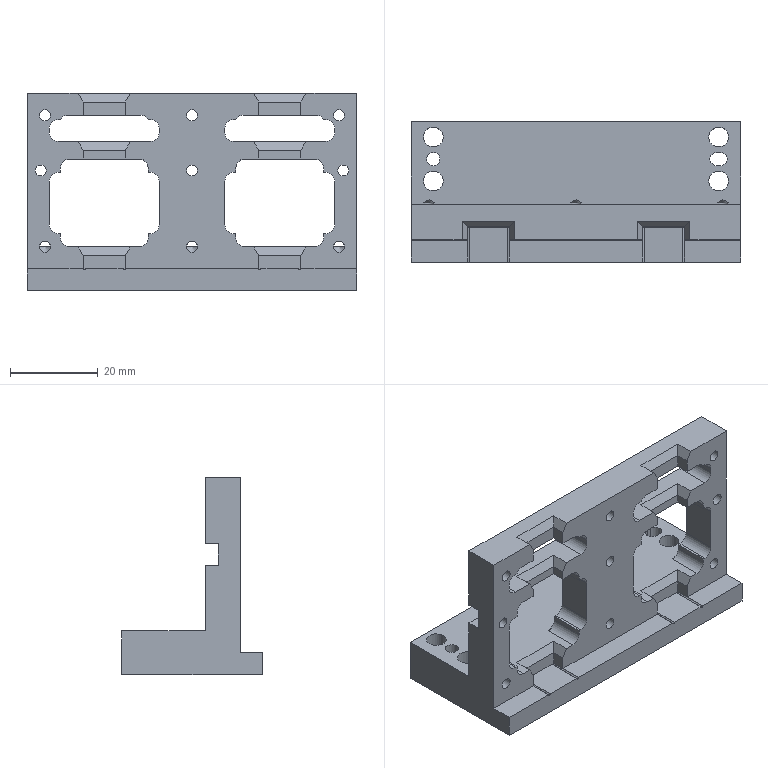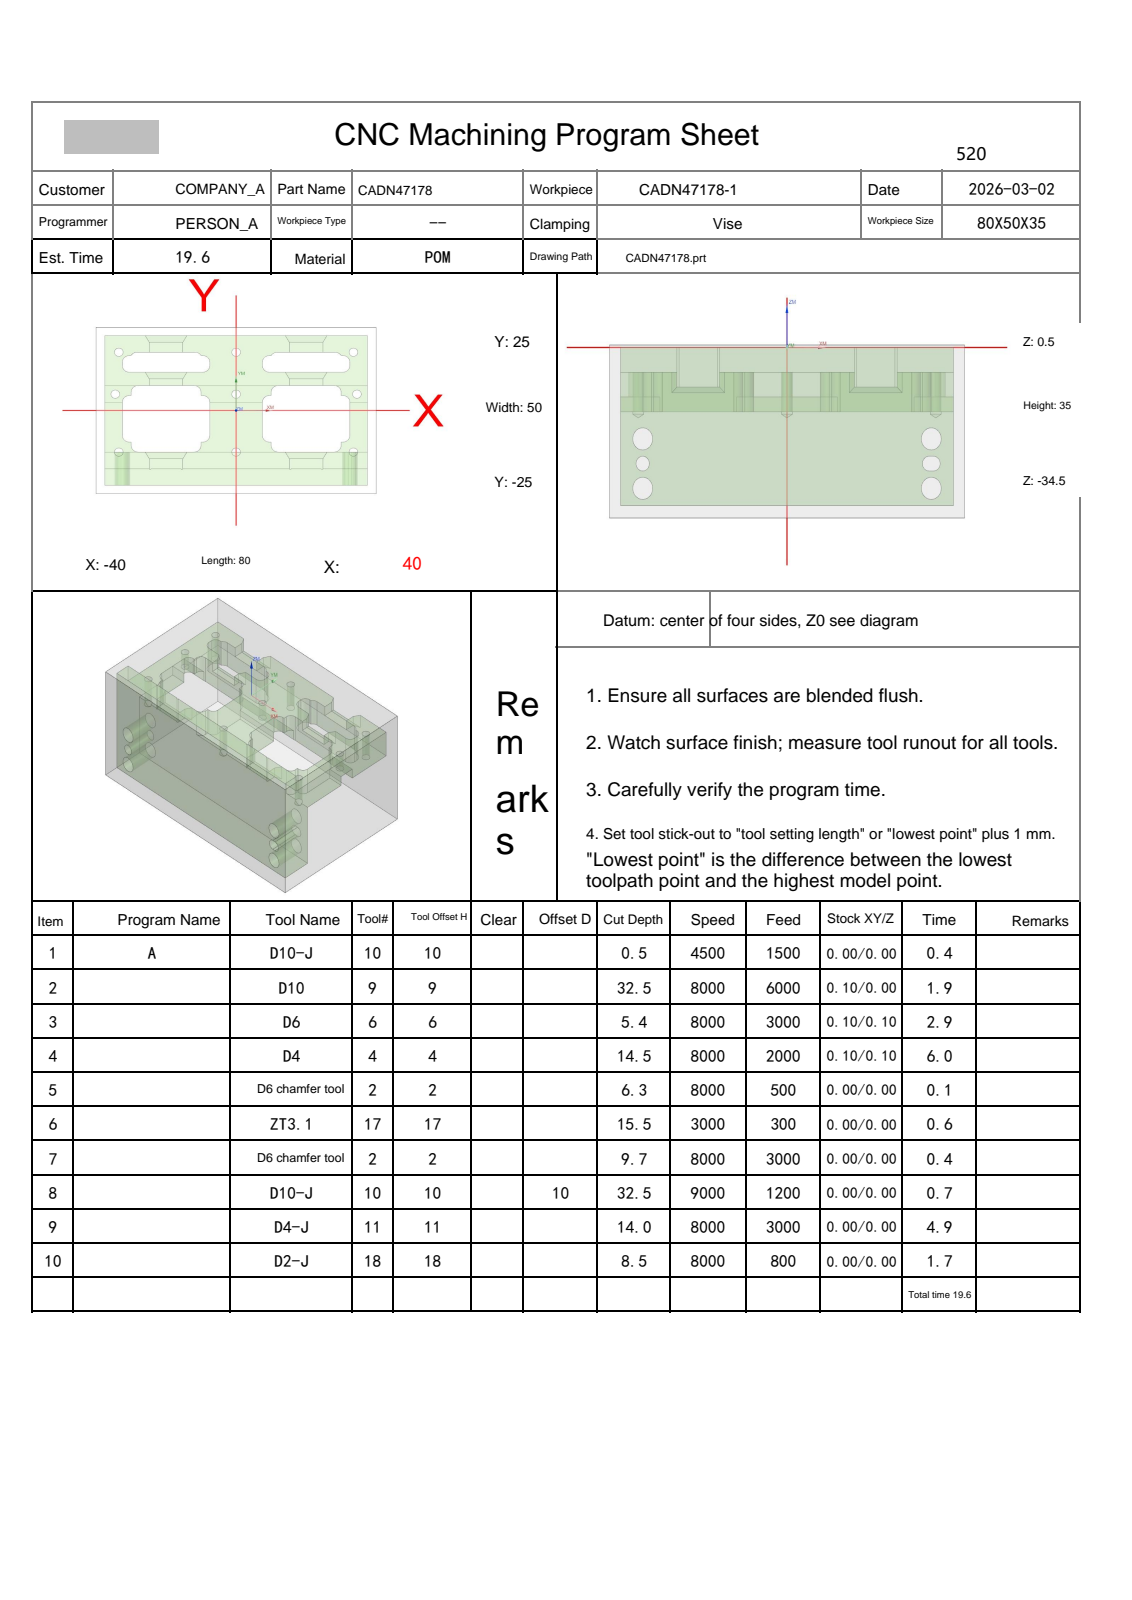NC program | NX | posted by the shop | part box 75 x 32 x 45 mm
Lines 8500 to 9882 of 18359:
N9 T11 M06
(D4-J  D=4. R=0. H=11 ce=0.40 di=0.00)
G00 G90 G54 X-40.3 Y7.17 M03 S7000
G43 H11 Z10.5
M08
Z-3.5
G01 Z-5. F1500.
X-38.7
G03 X-37.9 Y7.97 I0.0 J.8
G01 Y22.501
G02 X-37.501 Y22.9 I.4 J-.001
G01 X-25.954
G02 X-25.609 Y22.701 I-.001 J-.4
G01 X-24.453 Y20.699
G02 X-24.4 Y20.501 I-.347 J-.199
G01 Y17.499
G02 X-24.799 Y17.1 I-.4 J.001
G01 X-29.192
X-29.654 Y16.299
G02 X-29.999 Y16.1 I-.346 J.201
G01 X-32.1
Y11.9
X-25.954
G02 X-25.609 Y11.701 I-.001 J-.4
G01 X-24.453 Y9.699
G02 X-24.4 Y9.501 I-.347 J-.199
G01 Y7.499
G02 X-24.799 Y7.1 I-.4 J.001
G01 X-29.6
Y4.499
G02 X-29.999 Y4.1 I-.4 J.001
G01 X-32.1
Y-9.1
X-29.999
G02 X-29.6 Y-9.499 I-.001 J-.4
G01 Y-12.1
X-25.954
G02 X-25.609 Y-12.299 I-.001 J-.4
G01 X-24.453 Y-14.301
G02 X-24.4 Y-14.499 I-.347 J-.199
G01 Y-14.701
G02 X-24.799 Y-15.1 I-.4 J.001
G01 X-37.501
G02 X-37.9 Y-14.701 I.001 J.4
G01 Y8.805
G02 X-37.783 Y9.087 I.4 J0.0
G01 X-36.017 Y10.853
G03 X-35.9 Y11.135 I-.283 J.283
G01 Y20.501
G02 X-35.501 Y20.9 I.4 J-.001
G01 X-27.108
G02 X-26.764 Y20.701 I-.001 J-.4
G01 X-26.453 Y20.163
G02 X-26.4 Y19.965 I-.347 J-.199
G01 Y19.499
G02 X-26.799 Y19.1 I-.4 J.001
G01 X-29.192
G03 X-30.817 Y18.266 I0.0 J-2.
G02 X-31.14 Y18.1 I-.324 J.234
G01 X-32.1
G03 X-34.1 Y16.1 I0.0 J-2.
G01 Y11.9
G03 X-32.1 Y9.9 I2. J0.0
G01 X-27.108
G02 X-26.709 Y9.5 I-.001 J-.4
X-27.108 Y9.1 I-.4 J0.0
G01 X-29.6
G03 X-31.6 Y7.1 I0.0 J-2.
G01 Y6.499
G02 X-31.999 Y6.1 I-.4 J.001
G01 X-32.1
G03 X-34.1 Y4.1 I0.0 J-2.
G01 Y-9.1
G03 X-32.1 Y-11.1 I2. J0.0
G01 X-31.999
G02 X-31.6 Y-11.499 I-.001 J-.4
G01 Y-12.1
G03 X-31.536 Y-12.601 I2. J0.0
G01 X-31.524 Y-12.7
G02 X-31.923 Y-13.1 I-.4 J0.0
G01 X-35.501
G02 X-35.9 Y-12.701 I.001 J.4
G01 Y8.615
G02 X-35.66 Y8.855 I.24 J0.0
G01 X-35.571 Y8.838
X-34.132 Y8.263
G03 X-33.841 Y8.207 I.291 J.729
G01 X-33.729 Y8.215
X-33.673 Y8.225
X-33.622 Y8.201
G02 X-33.499 Y8.016 I-.077 J-.185
G01 X-33.503 Y7.973
X-33.515 Y7.918
X-33.526 Y7.865
X-33.56 Y7.823
X-33.611 Y7.804
X-33.678 Y7.776
X-33.74 Y7.763
G02 X-33.9 Y7.922 I0.0 J.16
G01 Y8.018
X-33.904 Y8.068
X-33.886 Y8.115
X-33.85 Y8.149
X-33.7 Y8.217
X-33.622 Y8.201
G02 X-33.499 Y8.016 I-.077 J-.185
G01 X-33.503 Y7.973
X-33.515 Y7.918
X-33.526 Y7.865
X-33.56 Y7.823
X-33.611 Y7.804
X-33.678 Y7.776
X-33.739 Y7.753
X-33.804 Y7.766
X-33.852 Y7.809
G03 X-34.414 Y8.039 I-.561 J-.57
X-34.984 Y7.801 I0.0 J-.8
G01 Z-3.5
G00 Z-1.
X11.818 Y14.3
Z-3.5
G01 Z-5.
X8.7 Y12.7
G03 X7.9 Y11.9 I0.0 J-.8
G01 X14.047
G02 X14.392 Y11.7 I-.001 J-.4
G01 X15.547 Y9.699
G02 X15.6 Y9.501 I-.347 J-.199
G01 Y7.499
G02 X15.201 Y7.1 I-.4 J.001
G01 X10.4
Y4.345
G02 X10.2 Y4.146 I-.2 J.001
G01 X10.059 Y4.204
X9.875 Y4.387
X7.9 Y3.569
Y-9.1
X10.001
G02 X10.4 Y-9.499 I-.001 J-.4
G01 Y-12.1
X14.047
G02 X14.391 Y-12.299 I-.001 J-.4
G01 X15.547 Y-14.301
G02 X15.6 Y-14.499 I-.347 J-.199
G01 Y-14.701
G02 X15.201 Y-15.1 I-.4 J.001
G01 X-15.201
G02 X-15.6 Y-14.701 I.001 J.4
G01 Y-14.499
G02 X-15.547 Y-14.301 I.4 J-.001
G01 X-14.391 Y-12.299
G02 X-14.047 Y-12.1 I.346 J-.201
G01 X-10.4
Y-9.499
G02 X-10.001 Y-9.1 I.4 J-.001
G01 X-7.9
Y3.489
X-9.122 Y4.1
X-10.001
G02 X-10.4 Y4.499 I.001 J.4
G01 Y7.1
X-15.201
G02 X-15.6 Y7.499 I.001 J.4
G01 Y9.501
G02 X-15.547 Y9.699 I.4 J-.001
G01 X-14.391 Y11.701
G02 X-14.047 Y11.9 I.346 J-.201
G01 X-7.9
Y16.1
X-10.001
G02 X-10.346 Y16.299 I.001 J.4
G01 X-10.808 Y17.1
X-15.201
G02 X-15.6 Y17.499 I.001 J.4
G01 Y20.501
G02 X-15.547 Y20.699 I.4 J-.001
G01 X-14.391 Y22.701
G02 X-14.047 Y22.9 I.346 J-.201
G01 X14.047
G02 X14.391 Y22.701 I-.001 J-.4
G01 X15.547 Y20.699
G02 X15.6 Y20.501 I-.347 J-.199
G01 Y17.499
G02 X15.201 Y17.1 I-.4 J.001
G01 X10.808
X10.346 Y16.299
G02 X10.001 Y16.1 I-.346 J.201
G01 X7.9
Y11.9
X9.9
G02 X10.276 Y11.635 I0.0 J-.4
G01 X10.805 Y10.165
G03 X11.181 Y9.9 I.376 J.135
G01 X12.892
G02 X13.291 Y9.5 I-.001 J-.4
X12.892 Y9.1 I-.4 J0.0
G01 X10.4
G03 X8.4 Y7.1 I0.0 J-2.
G01 Y6.207
G02 X8.154 Y5.839 I-.4 J.001
G01 X7.135 Y5.417
G03 X5.9 Y3.569 I.765 J-1.848
G01 Y-9.1
G03 X7.9 Y-11.1 I2. J0.0
G01 X8.001
G02 X8.4 Y-11.499 I-.001 J-.4
G01 Y-12.1
G03 X8.464 Y-12.601 I2. J0.0
G01 X8.476 Y-12.7
G02 X8.078 Y-13.1 I-.4 J0.0
G01 X-8.078
G02 X-8.476 Y-12.7 I.001 J.4
G01 X-8.464 Y-12.601
G03 X-8.4 Y-12.1 I-1.936 J.501
G01 Y-11.499
G02 X-8.001 Y-11.1 I.4 J-.001
G01 X-7.9
G03 X-5.9 Y-9.1 I0.0 J2.
G01 Y3.489
G03 X-7.006 Y5.278 I-2. J0.0
G01 X-8.18 Y5.865
G02 X-8.4 Y6.221 I.18 J.357
G01 Y7.1
G03 X-10.4 Y9.1 I-2. J0.0
G01 X-12.892
G02 X-13.291 Y9.5 I.001 J.4
X-12.892 Y9.9 I.4 J0.0
G01 X-7.9
G03 X-5.9 Y11.9 I0.0 J2.
G01 Y16.1
G03 X-7.9 Y18.1 I-2. J0.0
G01 X-8.86
G02 X-9.183 Y18.266 I.001 J.4
G03 X-10.808 Y19.1 I-1.625 J-1.166
G01 X-13.201
G02 X-13.6 Y19.499 I.001 J.4
G01 Y19.965
G02 X-13.547 Y20.163 I.4 J-.001
G01 X-13.236 Y20.701
G02 X-12.892 Y20.9 I.346 J-.201
G01 X12.892
G02 X13.236 Y20.701 I-.001 J-.4
G01 X13.547 Y20.163
G02 X13.6 Y19.965 I-.347 J-.199
G01 Y19.499
G02 X13.201 Y19.1 I-.4 J.001
G01 X10.808
G03 X9.183 Y18.266 I0.0 J-2.
G02 X8.86 Y18.1 I-.324 J.234
G01 X7.9
G03 X5.9 Y16.1 I0.0 J-2.
G01 Y11.9
G03 X7.9 Y9.9 I2. J0.0
G01 X8.504
G02 X8.664 Y9.74 I0.0 J-.16
G01 X8.615 Y9.625
X6.506 Y7.588
X6.455 Y7.546
X6.419 Y7.489
X6.403 Y7.425
G02 X6.195 Y7.187 I-.38 J.124
G03 X3.9 Y3.569 I1.705 J-3.618
G01 Y-9.1
G03 X4.174 Y-10.556 I4. J0.0
G01 X4.201 Y-10.7
G02 X3.803 Y-11.1 I-.4 J0.0
G01 X-3.803
G02 X-4.201 Y-10.7 I.001 J.4
G01 X-4.174 Y-10.556
G03 X-3.9 Y-9.1 I-3.726 J1.456
G01 Y3.489
G03 X-6.111 Y7.067 I-4. J0.0
G01 X-6.195 Y7.109
G02 X-6.414 Y7.431 I.18 J.357
G03 X-6.466 Y7.826 I-3.986 J-.331
G01 X-6.473 Y7.897
G02 X-6.24 Y8.261 I.4 J0.0
G03 X-3.9 Y11.9 I-1.66 J3.639
G01 Y16.1
G03 X-4.548 Y18.283 I-4. J0.0
G02 X-4.612 Y18.5 I.336 J.217
X-4.214 Y18.9 I.4 J0.0
G01 X4.214
G02 X4.612 Y18.5 I-.001 J-.4
X4.548 Y18.283 I-.4 J0.0
G03 X3.9 Y16.1 I3.352 J-2.183
G01 Y11.9
G03 X5.297 Y8.862 I4. J0.0
G02 X5.395 Y8.65 I-.182 J-.213
X5.265 Y8.413 I-.28 J0.0
G01 X3.006 Y6.983
X2.933 Y6.937
X2.886 Y6.865
G03 X1.9 Y3.569 I5.014 J-3.296
G01 Y-8.702
G02 X1.502 Y-9.1 I-.4 J.002
G01 X-1.502
G02 X-1.9 Y-8.702 I.002 J.4
G01 Y3.489
G03 X-3.378 Y7.433 I-6. J0.0
G02 X-3.476 Y7.694 I.302 J.262
X-3.378 Y7.956 I.4 J0.0
G03 X-1.9 Y11.9 I-4.522 J3.944
G01 Y16.1
G03 X-1.912 Y16.476 I-6. J0.0
G01 X-1.913 Y16.5
G02 X-1.514 Y16.9 I.4 J0.0
G01 X1.514
G02 X1.913 Y16.5 I-.002 J-.4
G01 X1.912 Y16.476
G03 X1.9 Y16.1 I5.988 J-.376
G01 Y11.9
G03 X2.706 Y8.897 I6. J0.0
G02 X2.759 Y8.696 I-.346 J-.2
X2.604 Y8.38 I-.4 J0.0
G01 X.678 Y6.897
G03 X.555 Y6.739 I.244 J-.317
X.255 Y5.924 I7.345 J-3.17
G02 X-.013 Y5.728 I-.267 J.084
X-.279 Y5.922 I0.0 J.28
G03 X-.976 Y7.496 I-7.621 J-2.433
G02 X-1.029 Y7.694 I.347 J.199
X-.976 Y7.893 I.4 J0.0
G03 X-.267 Y9.506 I-6.924 J4.007
G02 X0.0 Y9.7 I.267 J-.085
X.267 Y9.506 I0.0 J-.28
G03 X.954 Y7.932 I7.633 J2.394
G02 X1.006 Y7.74 I-.348 J-.197
G01 Y7.735
G02 X.954 Y7.538 I-.4 J0.0
G03 X.597 Y6.835 I6.946 J-3.968
X.527 Y6.508 I.73 J-.327
X1.001 Y5.778 I.8 J0.0
G01 Z-3.5
G00 Z-1.
X40.3 Y8.77
Z-3.5
G01 Z-5.
X38.7
G03 X37.9 Y7.97 I0.0 J-.8
G01 Y-14.701
G02 X37.501 Y-15.1 I-.4 J.001
G01 X24.799
G02 X24.4 Y-14.701 I.001 J.4
G01 Y-14.499
G02 X24.453 Y-14.301 I.4 J-.001
G01 X25.609 Y-12.299
G02 X25.954 Y-12.1 I.346 J-.201
G01 X29.6
Y-9.499
G02 X29.999 Y-9.1 I.4 J-.001
G01 X32.1
Y4.1
X29.999
G02 X29.6 Y4.499 I.001 J.4
G01 Y7.1
X24.799
G02 X24.4 Y7.5 I.001 J.4
G01 Y9.1
Y9.501
G02 X24.453 Y9.699 I.4 J-.001
G01 X25.609 Y11.701
G02 X25.954 Y11.9 I.346 J-.201
G01 X32.1
Y16.1
X29.999
G02 X29.654 Y16.299 I.001 J.4
G01 X29.192 Y17.1
X24.799
G02 X24.4 Y17.499 I.001 J.4
G01 Y20.501
G02 X24.453 Y20.699 I.4 J-.001
G01 X25.609 Y22.701
G02 X25.954 Y22.9 I.346 J-.201
G01 X37.501
G02 X37.9 Y22.501 I-.001 J-.4
G01 Y5.97
G02 X37.635 Y5.594 I-.4 J0.0
G01 X36.165 Y5.065
G03 X35.9 Y4.689 I.135 J-.376
G01 Y-12.701
G02 X35.501 Y-13.1 I-.4 J.001
G01 X31.923
G02 X31.524 Y-12.7 I.001 J.4
G01 X31.536 Y-12.601
G03 X31.6 Y-12.1 I-1.936 J.501
G01 Y-11.499
G02 X31.999 Y-11.1 I.4 J-.001
G01 X32.1
G03 X34.1 Y-9.1 I0.0 J2.
G01 Y4.1
G03 X32.1 Y6.1 I-2. J0.0
G01 X31.999
G02 X31.6 Y6.499 I.001 J.4
G01 Y7.1
G03 X29.6 Y9.1 I-2. J0.0
G01 X27.108
G02 X26.709 Y9.5 I.001 J.4
X27.108 Y9.9 I.4 J0.0
G01 X32.1
G03 X34.1 Y11.9 I0.0 J2.
G01 Y16.1
G03 X32.1 Y18.1 I-2. J0.0
G01 X31.14
G02 X30.817 Y18.266 I.001 J.4
G03 X29.192 Y19.1 I-1.625 J-1.166
G01 X26.799
G02 X26.4 Y19.499 I.001 J.4
G01 Y19.965
G02 X26.453 Y20.163 I.4 J-.001
G01 X26.764 Y20.701
G02 X27.108 Y20.9 I.346 J-.201
G01 X35.501
G02 X35.9 Y20.501 I-.001 J-.4
G01 Y7.329
G02 X35.66 Y7.089 I-.24 J0.0
G01 X35.568 Y7.107
X34.125 Y7.705
G03 X33.818 Y7.766 I-.307 J-.742
G01 X33.753 Y7.764
X33.713 Y7.755
X33.678 Y7.776
X33.611 Y7.804
X33.56 Y7.823
X33.526 Y7.865
X33.515 Y7.918
X33.503 Y7.973
X33.499 Y8.016
G02 X33.625 Y8.202 I.2 J0.0
G01 X33.7 Y8.217
G02 X33.9 Y8.018 I0.0 J-.2
G01 Y7.922
X33.905 Y7.881
X33.89 Y7.843
X33.859 Y7.816
X33.81 Y7.768
X33.742 Y7.753
X33.678 Y7.776
X33.611 Y7.804
X33.56 Y7.823
X33.526 Y7.865
X33.515 Y7.918
X33.503 Y7.973
X33.499 Y8.016
G02 X33.625 Y8.202 I.2 J0.0
G01 X33.7 Y8.217
X33.843 Y8.156
G03 X34.416 Y7.914 I.573 J.558
X34.975 Y8.141 I0.0 J.8
G01 Z-3.5
G00 Z10.5
G00 G90 X-38.119 Y-14.771 M03 S8000
Z5.5
Z-2.38
G01 Z-3.38 F800.
G41 D11
X-38.096 Y-14.969
G03 X-37.5 Y-15.5 I.596 J.069
G01 X-24.8
G02 X-24.55 Y-15.516 I0.0 J-2.
X-24.3 Y-15.5 I.25 J-1.984
G01 X-15.7
G02 X-15.45 Y-15.516 I0.0 J-2.
X-15.2 Y-15.5 I.25 J-1.984
G01 X15.2
G02 X15.45 Y-15.516 I0.0 J-2.
X15.7 Y-15.5 I.25 J-1.984
G01 X24.3
G02 X24.55 Y-15.516 I0.0 J-2.
G03 X25.078 Y-14.92 I-.072 J.596
G01 Y-14.9
G40 X25.071 Y-14.7
Z-2.38
G00 Z5.5
X-23.9 Y24.401
Z-5.76
G01 Z-6.76
G41 D11
X-24.061 Y24.282
G03 X-24.303 Y23.8 I.358 J-.482
X-24.223 Y23.5 I.6 J0.0
G01 X-23.068 Y21.5
G02 X-22.8 Y20.5 I-1.732 J-1.
G01 Y17.5
G02 X-24.8 Y15.5 I-2. J0.0
G01 X-24.808
X-28.268
G02 X-30. Y14.5 I-1.732 J1.
G01 X-30.5
Y13.5
X-25.955
X-25.879 Y13.499
G02 X-24.223 Y12.5 I-.075 J-1.999
G01 X-23.068 Y10.5
G02 X-22.8 Y9.5 I-1.732 J-1.
G01 Y7.5
G02 X-24.8 Y5.5 I-2. J0.0
G01 X-24.808
X-28.
Y4.5
G02 X-30. Y2.5 I-2. J0.0
G01 X-30.5
Y-7.5
X-30.
G02 X-28. Y-9.5 I0.0 J-2.
G01 Y-10.5
X-25.955
X-25.889 Y-10.501
G02 X-24.223 Y-11.5 I-.065 J-1.999
G01 X-23.068 Y-13.5
G02 X-22.8 Y-14.5 I-1.732 J-1.
G01 Y-15.5
X-17.2
Y-14.5
G02 X-16.932 Y-13.5 I2. J0.0
G01 X-15.777 Y-11.5
G02 X-14.045 Y-10.5 I1.732 J-1.
G01 X-12.
Y-9.5
G02 X-10. Y-7.5 I2. J0.0
G01 X-9.5
Y2.5
X-10.
G02 X-12. Y4.5 I0.0 J2.
G01 Y5.5
X-15.2
G02 X-17.2 Y7.5 I0.0 J2.
G01 Y9.5
G02 X-16.932 Y10.5 I2. J0.0
G01 X-15.777 Y12.5
G02 X-14.126 Y13.498 I1.732 J-1.
G01 X-14.045 Y13.5
X-9.5
Y14.5
X-10.
G02 X-11.732 Y15.5 I0.0 J2.
G01 X-15.2
G02 X-17.2 Y17.5 I0.0 J2.
G01 Y20.5
G02 X-16.932 Y21.5 I2. J0.0
G01 X-15.777 Y23.5
G03 X-15.697 Y23.8 I-.52 J.3
X-15.939 Y24.282 I-.6 J0.0
G01 G40 X-16.1 Y24.401
Z-5.76
G00 Z5.5
X-29.381 Y1.771
Z-9.14
G01 Z-10.14
G41 D11
X-29.404 Y1.969
G03 X-30. Y2.5 I-.596 J-.069
G01 X-30.5
Y-7.5
X-30.
G02 X-28. Y-9.5 I0.0 J-2.
G01 Y-10.5
X-12.
Y-9.5
G02 X-10. Y-7.5 I2. J0.0
G01 X-9.5
Y2.492
Y2.5
X-10.
G02 X-12. Y4.5 I0.0 J2.
G01 Y5.5
X-28.
Y4.5
G02 X-30. Y2.5 I-2. J0.0
G03 X-30.3 Y2.2 I0.0 J-.3
G01 G40 X-29.9 Y1.902
Z-9.14
G00 X-29.381 Y1.771
Z-12.52
G01 Z-13.52
G41 D11
X-29.404 Y1.969
G03 X-30. Y2.5 I-.596 J-.069
G01 X-30.5
Y-7.5
X-30.
G02 X-28. Y-9.5 I0.0 J-2.
G01 Y-10.5
X-12.
Y-9.5
G02 X-10. Y-7.5 I2. J0.0
G01 X-9.5
Y2.492
Y2.5
X-10.
G02 X-12. Y4.5 I0.0 J2.
G01 Y5.5
X-28.
Y4.5
G02 X-30. Y2.5 I-2. J0.0
G03 X-30.3 Y2.2 I0.0 J-.3
G01 G40 X-29.9 Y1.902
Z-12.52
G00 Z3.
X-28.821 Y14.189
Z-9.14
G01 Z-10.14
G41 D11
X-29.4 Y13.9
G03 X-30. Y14.5 I-.6 J0.0
G01 X-30.5
Y13.5
X-9.5
Y14.5
X-10.
G02 X-11.732 Y15.5 I0.0 J2.
G01 X-28.268
G02 X-30. Y14.5 I-1.732 J1.
G03 X-30.3 Y14.2 I0.0 J-.3
G01 G40 X-29. Y14.1
Z-9.14
G00 Z3.
X-23.252 Y-11.58
Z-7.
G01 Z-8.
G41 D11
X-23.426 Y-11.68
G03 X-23.726 Y-12.2 I.3 J-.52
X-23.645 Y-12.5 I.6 J0.0
G01 X-23.068 Y-13.5
G02 X-22.8 Y-14.5 I-1.732 J-1.
G01 Y-15.5
X-17.2
Y-14.5
G02 X-16.932 Y-13.5 I2. J0.0
G01 X-16.355 Y-12.5
G03 X-16.274 Y-12.2 I-.52 J.3
X-16.574 Y-11.68 I-.6 J0.0
G01 G40 X-16.748 Y-11.58
Z-7.
G00 Z3.
X-14.599 Y4.7
Z-7.
G01 Z-8.
G41 D11
Y4.9
G03 X-15.199 Y5.5 I-.6 J0.0
G02 X-17.2 Y7.5 I0.0 J2.
G01 Y9.5
G02 X-16.932 Y10.5 I2. J0.0
G01 X-16.355 Y11.5
G03 X-16.274 Y11.8 I-.52 J.3
X-16.574 Y12.32 I-.6 J0.0
G01 G40 X-16.748 Y12.42
Z-7.
G00 Z3.
X-23.252
Z-7.
G01 Z-8.
G41 D11
X-23.426 Y12.32
G03 X-23.726 Y11.8 I.3 J-.52
X-23.645 Y11.5 I.6 J0.0
G01 X-23.068 Y10.5
G02 X-22.8 Y9.5 I-1.732 J-1.
G01 Y7.5
G02 X-24.8 Y5.5 I-2. J0.0
G03 X-25.4 Y4.9 I0.0 J-.6
G01 G40 Y4.7
Z-7.
G00 Z3.
X-14.599 Y14.7
Z-7.
G01 Z-8.
G41 D11
Y14.9
G03 X-15.199 Y15.5 I-.6 J0.0
G02 X-17.2 Y17.5 I0.0 J2.
G01 Y20.5
G02 X-16.932 Y21.5 I2. J0.0
G01 X-16.355 Y22.5
G03 X-16.274 Y22.8 I-.52 J.3
X-16.574 Y23.32 I-.6 J0.0
G01 G40 X-16.748 Y23.42
Z-7.
G00 Z3.
X-23.252
Z-7.
G01 Z-8.
G41 D11
X-23.426 Y23.32
G03 X-23.726 Y22.8 I.3 J-.52
X-23.645 Y22.5 I.6 J0.0
G01 X-23.068 Y21.5
G02 X-22.8 Y20.5 I-1.732 J-1.
G01 Y17.5
G02 X-24.8 Y15.5 I-2. J0.0
G03 X-25.4 Y14.9 I0.0 J-.6
G01 G40 Y14.7
Z-7.
G00 Z3.
X-28.821 Y14.189
Z-12.52
G01 Z-13.52
G41 D11
X-29.4 Y13.9
G03 X-30. Y14.5 I-.6 J0.0
G01 X-30.5
Y13.5
X-9.512
X-9.5
Y14.5
X-10.
G02 X-11.732 Y15.5 I0.0 J2.
G01 X-28.268
G02 X-30. Y14.5 I-1.732 J1.
G03 X-30.3 Y14.2 I0.0 J-.3
G01 G40 X-29. Y14.1
Z-12.52
G00 Z3.
X16.1 Y24.401
Z-5.76
G01 Z-6.76
G41 D11
X15.939 Y24.282
G03 X15.697 Y23.8 I.358 J-.482
X15.777 Y23.5 I.6 J0.0
G01 X16.932 Y21.5
G02 X17.2 Y20.5 I-1.732 J-1.
G01 Y17.5
G02 X15.2 Y15.5 I-2. J0.0
G01 X11.732
G02 X10. Y14.5 I-1.732 J1.
G01 X9.5
Y13.5
X14.045
X14.126 Y13.498
G02 X15.777 Y12.5 I-.081 J-1.998
G01 X16.932 Y10.5
G02 X17.2 Y9.5 I-1.732 J-1.
G01 Y7.5
G02 X15.2 Y5.5 I-2. J0.0
G01 X12.
Y4.5
G02 X10. Y2.5 I-2. J0.0
G01 X9.5
Y-7.5
X10.
G02 X12. Y-9.5 I0.0 J-2.
G01 Y-10.5
X14.045
G02 X15.777 Y-11.5 I0.0 J-2.
G01 X16.932 Y-13.5
G02 X17.2 Y-14.5 I-1.732 J-1.
G01 Y-15.5
X22.8
Y-14.5
G02 X23.068 Y-13.5 I2. J0.0
G01 X24.223 Y-11.5
G02 X25.907 Y-10.501 I1.732 J-1.
G01 X25.955 Y-10.5
X28.
Y-9.5
G02 X30. Y-7.5 I2. J0.0
G01 X30.5
Y2.5
X30.
G02 X28. Y4.5 I0.0 J2.
G01 Y5.5
X24.8
G02 X22.8 Y7.5 I0.0 J2.
G01 Y9.5
G02 X23.068 Y10.5 I2. J0.0
G01 X24.223 Y12.5
G02 X25.882 Y13.499 I1.732 J-1.
G01 X25.955 Y13.5
X30.5
Y14.5
X30.
G02 X28.268 Y15.5 I0.0 J2.
G01 X24.8
G02 X22.8 Y17.5 I0.0 J2.
G01 Y20.5
G02 X23.068 Y21.5 I2. J0.0
G01 X24.223 Y23.5
G03 X24.303 Y23.8 I-.52 J.3
X24.061 Y24.282 I-.6 J0.0
G01 G40 X23.9 Y24.401
Z-5.76
G00 Z5.5
X-17.8 Y-14.7
Z-4.
G01 Z-5.
G41 D11
Y-14.9
G03 X-17.2 Y-15.5 I.6 J0.0
G01 X-15.7
G02 X-15.45 Y-15.516 I0.0 J-2.
X-15.2 Y-15.5 I.25 J-1.984
G01 X15.2
G02 X15.45 Y-15.516 I0.0 J-2.
X15.7 Y-15.5 I.25 J-1.984
G01 X17.2
G03 X17.8 Y-14.9 I0.0 J.6
G01 G40 Y-14.7
Z-4.
G00 Z5.5
X29.381 Y-6.771
Z-9.14
G01 Z-10.14
G41 D11
X29.404 Y-6.969
G03 X30. Y-7.5 I.596 J.069
G01 X30.5
Y2.5
X30.
G02 X28. Y4.5 I0.0 J2.
G01 Y5.5
X12.
Y4.5
G02 X10. Y2.5 I-2. J0.0
G01 X9.5
Y-7.5
X10.
G02 X12. Y-9.5 I0.0 J-2.
G01 Y-10.5
X28.
Y-9.5
G02 X30. Y-7.5 I2. J0.0
G03 X30.3 Y-7.2 I0.0 J.3
G01 G40 X29.9 Y-6.902
Z-9.14
G00 X29.381 Y-6.771
Z-12.52
G01 Z-13.52
G41 D11
X29.404 Y-6.969
G03 X30. Y-7.5 I.596 J.069
G01 X30.5
Y2.4
X30.503 Y2.5
X30.
G02 X28. Y4.5 I0.0 J2.
G01 Y5.5
X12.008
X12.
Y4.5
G02 X10. Y2.5 I-2. J0.0
G01 X9.5
Y-7.5
X10.
G02 X12. Y-9.5 I0.0 J-2.
G01 Y-10.5
X28.
Y-9.5
G02 X30. Y-7.5 I2. J0.0
G03 X30.3 Y-7.2 I0.0 J.3
G01 G40 X29.9 Y-6.902
Z-12.52
G00 Z3.
X11.179 Y14.189
Z-9.14
G01 Z-10.14
G41 D11
X10.6 Y13.9
G03 X10. Y14.5 I-.6 J0.0
G01 X9.5
Y13.5
X30.5
Y14.5
X30.
G02 X28.268 Y15.5 I0.0 J2.
G01 X11.732
G02 X10. Y14.5 I-1.732 J1.
G03 X9.7 Y14.2 I0.0 J-.3
G01 G40 X11. Y14.1
Z-9.14
G00 Z3.
X16.748 Y-11.58
Z-7.
G01 Z-8.
G41 D11
X16.574 Y-11.68
G03 X16.274 Y-12.2 I.3 J-.52
X16.355 Y-12.5 I.6 J0.0
G01 X16.932 Y-13.5
G02 X17.2 Y-14.5 I-1.732 J-1.
G01 Y-15.5
X22.8
Y-14.5
G02 X23.068 Y-13.5 I2. J0.0
G01 X23.645 Y-12.5
G03 X23.726 Y-12.2 I-.52 J.3
X23.426 Y-11.68 I-.6 J0.0
G01 G40 X23.252 Y-11.58
Z-7.
G00 Z3.
X16.748 Y12.42
Z-7.
G01 Z-8.
G41 D11
X16.574 Y12.32
G03 X16.274 Y11.8 I.3 J-.52
X16.355 Y11.5 I.6 J0.0
G01 X16.932 Y10.5
G02 X17.2 Y9.5 I-1.732 J-1.
G01 Y7.5
G02 X15.2 Y5.5 I-2. J0.0
G03 X14.599 Y4.9 I0.0 J-.6
G01 G40 Y4.7
Z-7.
G00 Z3.
X25.4
Z-7.
G01 Z-8.
G41 D11
Y4.9
G03 X24.8 Y5.5 I-.6 J0.0
G02 X22.8 Y7.5 I0.0 J2.
G01 Y9.5
G02 X23.068 Y10.5 I2. J0.0
G01 X23.645 Y11.5
G03 X23.726 Y11.8 I-.52 J.3
X23.426 Y12.32 I-.6 J0.0
G01 G40 X23.252 Y12.42
Z-7.
G00 Z3.
X16.748 Y23.42
Z-7.
G01 Z-8.
G41 D11
X16.574 Y23.32
G03 X16.274 Y22.8 I.3 J-.52
X16.355 Y22.5 I.6 J0.0
G01 X16.932 Y21.5
G02 X17.2 Y20.5 I-1.732 J-1.
G01 Y17.5
G02 X15.2 Y15.5 I-2. J0.0
G03 X14.599 Y14.9 I0.0 J-.6
G01 G40 Y14.7
Z-7.
G00 Z3.
X25.4
Z-7.
G01 Z-8.
G41 D11
Y14.9
G03 X24.8 Y15.5 I-.6 J0.0
G02 X22.8 Y17.5 I0.0 J2.
G01 Y20.5
G02 X23.068 Y21.5 I2. J0.0
G01 X23.645 Y22.5
G03 X23.726 Y22.8 I-.52 J.3
X23.426 Y23.32 I-.6 J0.0
G01 G40 X23.252 Y23.42
Z-7.
G00 Z3.
X11.179 Y14.189
Z-12.52
G01 Z-13.52
G41 D11
X10.6 Y13.9
G03 X10. Y14.5 I-.6 J0.0
G01 X9.5
Y13.5
X30.493
X30.5
Y14.5
X30.
G02 X28.268 Y15.5 I0.0 J2.
G01 X11.732
G02 X10. Y14.5 I-1.732 J1.
G03 X9.7 Y14.2 I0.0 J-.3
G01 G40 X11. Y14.1
Z-12.52
G00 Z5.5
G00 G90 X-20.8 Y23.3 M03 S7000
Z10.5
Z-6.5
G01 Z-8. F1500.
Y21.7
G03 X-20. Y20.9 I.8 J0.0
G01 X-17.999
G02 X-17.6 Y20.501 I-.001 J-.4
G01 Y7.499
G02 X-17.999 Y7.1 I-.4 J.001
G01 X-22.001
G02 X-22.4 Y7.499 I.001 J.4
G01 Y20.501
G02 X-22.001 Y20.9 I.4 J-.001
G01 X-18.
G02 X-17.6 Y20.5 I0.0 J-.4
X-17.687 Y20.251 I-.4 J0.0
G01 X-19.513 Y17.96
G03 X-19.6 Y17.711 I.313 J-.249
G01 Y9.499
G02 X-20. Y9.1 I-.4 J.001
X-20.4 Y9.499 I0.0 J.4
G01 Y18.501
G02 X-20. Y18.9 I.4 J-.001
X-19.744 Y18.807 I0.0 J-.4
X-19.6 Y18.501 I-.256 J-.307
G01 Y17.85
G03 X-18.8 Y17.05 I.8 J0.0
G01 Z-6.5
G00 Z10.5
X19.2 Y23.3
Z-6.5
G01 Z-8.
Y21.7
G03 X20. Y20.9 I.8 J0.0
G01 X22.001
G02 X22.4 Y20.501 I-.001 J-.4
G01 Y7.499
G02 X22.001 Y7.1 I-.4 J.001
G01 X17.999
G02 X17.6 Y7.499 I.001 J.4
G01 Y20.501
G02 X17.999 Y20.9 I.4 J-.001
G01 X22.
G02 X22.4 Y20.5 I0.0 J-.4
X22.313 Y20.251 I-.4 J0.0
G01 X20.487 Y17.96
G03 X20.4 Y17.711 I.313 J-.249
G01 Y9.499
G02 X20. Y9.1 I-.4 J.001
X19.6 Y9.499 I0.0 J.4
G01 Y18.501
G02 X20. Y18.9 I.4 J-.001
X20.256 Y18.807 I0.0 J-.4
X20.4 Y18.501 I-.256 J-.307
G01 Y17.85
G03 X21.2 Y17.05 I.8 J0.0
G01 Z-6.5
G00 Z10.5
G00 G90 X-38.119 Y-14.771 M03 S8000
Z5.5
Z-4.
G01 Z-5. F800.
G41 D11
X-38.096 Y-14.969
G03 X-37.5 Y-15.5 I.596 J.069
G01 X-24.8
G02 X-24.55 Y-15.516 I0.0 J-2.
X-24.3 Y-15.5 I.25 J-1.984
G01 X-15.7
G02 X-15.45 Y-15.516 I0.0 J-2.
X-15.2 Y-15.5 I.25 J-1.984
G01 X15.2
G02 X15.45 Y-15.516 I0.0 J-2.
X15.7 Y-15.5 I.25 J-1.984
G01 X24.3
G02 X24.55 Y-15.516 I0.0 J-2.
X24.8 Y-15.5 I.25 J-1.984
G01 X37.5
G03 X38.096 Y-14.969 I0.0 J.6
G01 G40 X38.119 Y-14.771
Z-4.
G00 Z5.5
G00 G90 X-23.647 Y11.523 M03 S8000
Z10.5
Z-7.5
G01 Z-8.008 F3000.
X-16.353
X-16.345 Y11.536 Z-8.015
X-23.655
X-23.662 Y11.549 Z-8.023
X-16.338
X-16.33 Y11.562 Z-8.03
X-23.67
X-23.677 Y11.575 Z-8.038
X-16.323
X-16.315 Y11.588 Z-8.045
X-23.685
X-23.692 Y11.601 Z-8.053
X-16.308
X-16.3 Y11.614 Z-8.06
X-23.7
X-23.707 Y11.627 Z-8.068
X-16.293
X-16.285 Y11.64 Z-8.075
X-23.715
X-23.722 Y11.653 Z-8.083
X-16.278
X-16.27 Y11.666 Z-8.09
X-23.73
X-23.737 Y11.679 Z-8.098
X-16.263
X-16.255 Y11.692 Z-8.105
X-23.745
X-23.752 Y11.705 Z-8.113
X-16.248
X-16.24 Y11.718 Z-8.12
X-23.76
X-23.767 Y11.731 Z-8.128
X-16.233
X-16.225 Y11.744 Z-8.135
X-23.775
X-23.782 Y11.757 Z-8.143
X-16.218
X-16.21 Y11.77 Z-8.15
X-23.79
X-23.797 Y11.783 Z-8.158
X-16.203
X-16.195 Y11.796 Z-8.165
X-23.805
X-23.812 Y11.809 Z-8.173
X-16.188
X-16.18 Y11.822 Z-8.18
X-23.82
X-23.827 Y11.835 Z-8.188
X-16.173
X-16.165 Y11.848 Z-8.195
X-23.835
X-23.842 Y11.861 Z-8.203
X-16.158
X-16.15 Y11.874 Z-8.21
X-23.85
X-23.857 Y11.887 Z-8.218
X-16.143
X-16.135 Y11.9 Z-8.225
X-23.865
X-23.872 Y11.913 Z-8.233
X-16.128
X-16.12 Y11.926 Z-8.24
X-23.88
X-23.887 Y11.939 Z-8.248
X-16.113
X-16.105 Y11.952 Z-8.255
X-23.895
X-23.902 Y11.965 Z-8.263
X-16.098
X-16.09 Y11.978 Z-8.27
X-23.91
X-23.917 Y11.991 Z-8.278
X-16.083
X-16.075 Y12.004 Z-8.285
X-23.925
X-23.932 Y12.017 Z-8.293
X-16.068
X-16.06 Y12.03 Z-8.3
X-23.94
X-23.947 Y12.043 Z-8.308
X-16.053
X-16.045 Y12.056 Z-8.315
X-23.955
X-23.962 Y12.069 Z-8.323
X-16.038
X-16.03 Y12.082 Z-8.33
X-23.97
X-23.977 Y12.095 Z-8.338
X-16.023
X-16.015 Y12.108 Z-8.345
X-23.985
X-23.992 Y12.121 Z-8.353
X-16.008
X-16. Y12.134 Z-8.36
X-24.
X-24.007 Y12.147 Z-8.368
X-15.993
X-15.985 Y12.16 Z-8.375
X-24.015
X-24.022 Y12.173 Z-8.383
X-15.978
X-15.97 Y12.186 Z-8.39
X-24.03
X-24.037 Y12.198 Z-8.398
X-15.963
X-15.955 Y12.211 Z-8.405
X-24.045
X-24.052 Y12.224 Z-8.413
X-15.948
X-15.94 Y12.237 Z-8.42
X-24.06
X-24.067 Y12.25 Z-8.428
X-15.933
X-15.925 Y12.263 Z-8.435
X-24.075
X-24.082 Y12.276 Z-8.443
X-15.918
X-15.91 Y12.289 Z-8.45
X-24.09
X-24.112 Y12.302 Z-8.458
X-15.888
X-15.882 Y12.315 Z-8.465
X-24.118
X-24.123 Y12.328 Z-8.473
X-15.877
X-15.871 Y12.341 Z-8.48
X-24.129
X-24.135 Y12.354 Z-8.488
X-15.865
X-15.859 Y12.367 Z-8.495
X-24.141
X-24.148 Y12.38 Z-8.503
X-15.852
X-15.846 Y12.393 Z-8.51
X-24.154
X-24.161 Y12.406 Z-8.518
X-15.839
X-15.833 Y12.419 Z-8.525
X-24.167
X-24.174 Y12.432 Z-8.533
X-15.826
X-15.819 Y12.445 Z-8.54
X-24.181
X-24.188 Y12.458 Z-8.548
X-15.812
X-15.805 Y12.471 Z-8.555
X-24.195
X-24.202 Y12.484 Z-8.563
X-15.798
X-15.79 Y12.497 Z-8.57
X-24.21
X-24.217 Y12.51 Z-8.578
X-15.783
X-15.775 Y12.523 Z-8.585
X-24.225
X-24.232 Y12.536 Z-8.593
X-15.768
X-15.76 Y12.549 Z-8.6
X-24.24
X-24.248 Y12.562 Z-8.608
X-15.752
X-15.744 Y12.575 Z-8.615
X-24.256
X-24.265 Y12.588 Z-8.623
X-15.735
X-15.727 Y12.601 Z-8.63
X-24.273
X-24.282 Y12.614 Z-8.638
X-15.718
X-15.71 Y12.627 Z-8.645
X-24.29
X-24.299 Y12.64 Z-8.653
X-15.701
X-15.692 Y12.653 Z-8.66
X-24.308
X-24.318 Y12.666 Z-8.668
X-15.682
X-15.673 Y12.679 Z-8.675
X-24.327
X-24.336 Y12.692 Z-8.683
X-15.664
X-15.654 Y12.705 Z-8.69
X-24.346
X-24.356 Y12.718 Z-8.698
X-15.644
X-15.634 Y12.731 Z-8.705
X-24.366
X-24.376 Y12.744 Z-8.713
X-15.624
X-15.614 Y12.757 Z-8.72
X-24.386
X-24.397 Y12.77 Z-8.728
X-15.603
X-15.593 Y12.783 Z-8.735
X-24.407
X-24.418 Y12.796 Z-8.743
X-15.582
X-15.571 Y12.809 Z-8.75
X-24.429
X-24.441 Y12.822 Z-8.758
X-15.559
X-15.548 Y12.835 Z-8.765
X-24.452
X-24.464 Y12.848 Z-8.773
X-15.536
X-15.524 Y12.861 Z-8.78
X-24.476
X-24.488 Y12.874 Z-8.788
X-15.512
X-15.5 Y12.887 Z-8.795
X-24.5
X-24.512 Y12.9 Z-8.803
X-15.488
X-15.475 Y12.913 Z-8.81
X-24.525
X-24.538 Y12.926 Z-8.818
X-15.462
X-15.449 Y12.939 Z-8.825
X-24.551
X-24.565 Y12.952 Z-8.833
X-15.435
X-15.422 Y12.965 Z-8.84
X-24.578
X-24.592 Y12.978 Z-8.848
X-15.408
X-15.393 Y12.991 Z-8.855
X-24.607
X-24.621 Y13.004 Z-8.863
X-15.379
X-15.364 Y13.017 Z-8.87
X-24.636
X-24.651 Y13.03 Z-8.878
X-15.349
X-15.334 Y13.043 Z-8.885
X-24.666
X-24.682 Y13.056 Z-8.893
X-15.318
X-15.302 Y13.069 Z-8.9
X-24.698
X-24.715 Y13.082 Z-8.908
X-15.285
X-15.269 Y13.095 Z-8.915
X-24.731
X-24.748 Y13.108 Z-8.923
X-15.252
X-15.234 Y13.121 Z-8.93
X-24.766
X-24.784 Y13.134 Z-8.938
X-15.216
X-15.198 Y13.147 Z-8.945
X-24.802
X-24.821 Y13.16 Z-8.953
X-15.179
X-15.16 Y13.173 Z-8.96
X-24.84
X-24.86 Y13.186 Z-8.968
X-15.14
X-15.12 Y13.199 Z-8.975
X-24.88
X-24.901 Y13.212 Z-8.983
X-15.099
X-15.077 Y13.225 Z-8.99
X-24.923
X-24.945 Y13.238 Z-8.998
X-15.055
X-15.033 Y13.251 Z-9.005
X-24.967
X-24.991 Y13.264 Z-9.013
X-15.009
X-14.985 Y13.277 Z-9.02
X-25.015
X-25.04 Y13.29 Z-9.028
X-14.96
X-14.934 Y13.303 Z-9.035
X-25.066
X-25.092 Y13.316 Z-9.043
X-14.908
X-14.88 Y13.329 Z-9.05
X-25.12
X-25.149 Y13.342 Z-9.058
X-14.851
X-14.82 Y13.355 Z-9.065
X-25.18
X-25.212 Y13.368 Z-9.073
X-14.788
X-14.755 Y13.381 Z-9.08
X-25.245
X-25.281 Y13.394 Z-9.088
X-14.719
X-14.682 Y13.407 Z-9.095
X-25.318
X-25.359 Y13.42 Z-9.103
X-14.641
X-14.598 Y13.433 Z-9.11
X-25.402
X-25.45 Y13.446 Z-9.118
X-14.55
X-14.497 Y13.459 Z-9.125
X-25.503
X-25.563 Y13.472 Z-9.133
X-14.437
X-14.364 Y13.485 Z-9.14
X-25.636
X-25.77 Y13.502 Z-9.147
X-25.905 Y13.509 Z-9.155
X-14.095
G00 Z10.5
X16.353 Y11.523
Z-7.5
G01 Z-8.008
X23.647
X23.655 Y11.536 Z-8.015
X16.345
X16.338 Y11.549 Z-8.023
X23.662
X23.67 Y11.562 Z-8.03
X16.33
X16.323 Y11.575 Z-8.038
X23.677
X23.685 Y11.588 Z-8.045
X16.315
X16.308 Y11.601 Z-8.053
X23.692
X23.7 Y11.614 Z-8.06
X16.3